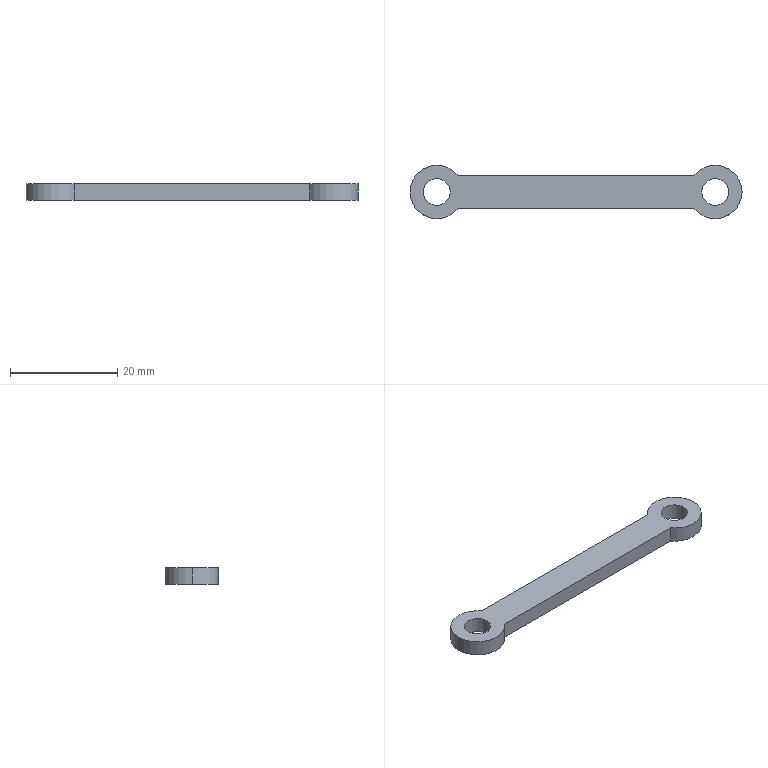Part | SolidWorks | features Extrusion 1 | 1 solid | 11 faces | box 62 x 10 x 3 mm | volume 1121 mm3 | cylinder 7 | plane 4 | commonest cylinder face diameters 5 x4 10 x3
STEP:
#1=CARTESIAN_POINT('',(49.5,0.,3.));
#2=VERTEX_POINT('',#1);
#3=CARTESIAN_POINT('',(54.5,0.,3.));
#4=VERTEX_POINT('',#3);
#5=CARTESIAN_POINT('',(52.,0.,3.));
#6=DIRECTION('',(0.,0.,1.));
#7=DIRECTION('',(1.,0.,0.));
#8=AXIS2_PLACEMENT_3D('',#5,#6,#7);
#9=CIRCLE('',#8,2.5);
#10=EDGE_CURVE('',#2,#4,#9,.T.);
#11=ORIENTED_EDGE('',*,*,#10,.T.);
#12=CARTESIAN_POINT('',(54.5,0.,0.));
#13=VERTEX_POINT('',#12);
#14=CARTESIAN_POINT('',(54.5,0.,3.));
#15=DIRECTION('',(0.,0.,-1.));
#16=VECTOR('',#15,1000.);
#17=LINE('',#14,#16);
#18=EDGE_CURVE('',#4,#13,#17,.T.);
#19=ORIENTED_EDGE('',*,*,#18,.T.);
#20=CARTESIAN_POINT('',(49.5,0.,0.));
#21=VERTEX_POINT('',#20);
#22=CARTESIAN_POINT('',(52.,0.,0.));
#23=DIRECTION('',(0.,0.,1.));
#24=DIRECTION('',(1.,0.,0.));
#25=AXIS2_PLACEMENT_3D('',#22,#23,#24);
#26=CIRCLE('',#25,2.5);
#27=EDGE_CURVE('',#21,#13,#26,.T.);
#28=ORIENTED_EDGE('',*,*,#27,.F.);
#29=CARTESIAN_POINT('',(49.5,0.,3.));
#30=DIRECTION('',(0.,0.,-1.));
#31=VECTOR('',#30,1000.);
#32=LINE('',#29,#31);
#33=EDGE_CURVE('',#2,#21,#32,.T.);
#34=ORIENTED_EDGE('',*,*,#33,.F.);
#35=EDGE_LOOP('',(#11,#19,#28,#34));
#36=FACE_OUTER_BOUND('',#35,.T.);
#37=CARTESIAN_POINT('',(52.,0.,3.));
#38=DIRECTION('',(0.,0.,-1.));
#39=DIRECTION('',(-1.,0.,0.));
#40=AXIS2_PLACEMENT_3D('',#37,#38,#39);
#41=CYLINDRICAL_SURFACE('',#40,2.5);
#42=ADVANCED_FACE('',(#36),#41,.F.);
#43=CARTESIAN_POINT('',(-2.5,0.,3.));
#44=VERTEX_POINT('',#43);
#45=CARTESIAN_POINT('',(2.5,0.,3.));
#46=VERTEX_POINT('',#45);
#47=CARTESIAN_POINT('',(0.,0.,3.));
#48=DIRECTION('',(0.,0.,1.));
#49=DIRECTION('',(1.,0.,0.));
#50=AXIS2_PLACEMENT_3D('',#47,#48,#49);
#51=CIRCLE('',#50,2.5);
#52=EDGE_CURVE('',#44,#46,#51,.T.);
#53=ORIENTED_EDGE('',*,*,#52,.T.);
#54=CARTESIAN_POINT('',(2.5,0.,0.));
#55=VERTEX_POINT('',#54);
#56=CARTESIAN_POINT('',(2.5,0.,3.));
#57=DIRECTION('',(0.,0.,-1.));
#58=VECTOR('',#57,1000.);
#59=LINE('',#56,#58);
#60=EDGE_CURVE('',#46,#55,#59,.T.);
#61=ORIENTED_EDGE('',*,*,#60,.T.);
#62=CARTESIAN_POINT('',(-2.5,0.,0.));
#63=VERTEX_POINT('',#62);
#64=CARTESIAN_POINT('',(0.,0.,0.));
#65=DIRECTION('',(0.,0.,1.));
#66=DIRECTION('',(1.,0.,0.));
#67=AXIS2_PLACEMENT_3D('',#64,#65,#66);
#68=CIRCLE('',#67,2.5);
#69=EDGE_CURVE('',#63,#55,#68,.T.);
#70=ORIENTED_EDGE('',*,*,#69,.F.);
#71=CARTESIAN_POINT('',(-2.5,0.,3.));
#72=DIRECTION('',(0.,0.,-1.));
#73=VECTOR('',#72,1000.);
#74=LINE('',#71,#73);
#75=EDGE_CURVE('',#44,#63,#74,.T.);
#76=ORIENTED_EDGE('',*,*,#75,.F.);
#77=EDGE_LOOP('',(#53,#61,#70,#76));
#78=FACE_OUTER_BOUND('',#77,.T.);
#79=CARTESIAN_POINT('',(0.,0.,3.));
#80=DIRECTION('',(0.,0.,-1.));
#81=DIRECTION('',(-1.,0.,0.));
#82=AXIS2_PLACEMENT_3D('',#79,#80,#81);
#83=CYLINDRICAL_SURFACE('',#82,2.5);
#84=ADVANCED_FACE('',(#78),#83,.F.);
#85=CARTESIAN_POINT('',(-5.,0.,3.));
#86=VERTEX_POINT('',#85);
#87=CARTESIAN_POINT('',(4.,-3.,3.));
#88=VERTEX_POINT('',#87);
#89=CARTESIAN_POINT('',(0.,0.,3.));
#90=DIRECTION('',(0.,0.,1.));
#91=DIRECTION('',(1.,0.,0.));
#92=AXIS2_PLACEMENT_3D('',#89,#90,#91);
#93=CIRCLE('',#92,5.);
#94=EDGE_CURVE('',#86,#88,#93,.T.);
#95=ORIENTED_EDGE('',*,*,#94,.F.);
#96=CARTESIAN_POINT('',(-5.,0.,0.));
#97=VERTEX_POINT('',#96);
#98=CARTESIAN_POINT('',(-5.,0.,3.));
#99=DIRECTION('',(0.,0.,-1.));
#100=VECTOR('',#99,1000.);
#101=LINE('',#98,#100);
#102=EDGE_CURVE('',#86,#97,#101,.T.);
#103=ORIENTED_EDGE('',*,*,#102,.T.);
#104=CARTESIAN_POINT('',(4.,-3.,0.));
#105=VERTEX_POINT('',#104);
#106=CARTESIAN_POINT('',(0.,0.,0.));
#107=DIRECTION('',(0.,0.,1.));
#108=DIRECTION('',(1.,0.,0.));
#109=AXIS2_PLACEMENT_3D('',#106,#107,#108);
#110=CIRCLE('',#109,5.);
#111=EDGE_CURVE('',#97,#105,#110,.T.);
#112=ORIENTED_EDGE('',*,*,#111,.T.);
#113=CARTESIAN_POINT('',(4.,-3.,3.));
#114=DIRECTION('',(0.,0.,-1.));
#115=VECTOR('',#114,1000.);
#116=LINE('',#113,#115);
#117=EDGE_CURVE('',#88,#105,#116,.T.);
#118=ORIENTED_EDGE('',*,*,#117,.F.);
#119=EDGE_LOOP('',(#95,#103,#112,#118));
#120=FACE_OUTER_BOUND('',#119,.T.);
#121=CARTESIAN_POINT('',(0.,0.,3.));
#122=DIRECTION('',(0.,0.,-1.));
#123=DIRECTION('',(-1.,0.,0.));
#124=AXIS2_PLACEMENT_3D('',#121,#122,#123);
#125=CYLINDRICAL_SURFACE('',#124,5.);
#126=ADVANCED_FACE('',(#120),#125,.T.);
#127=ORIENTED_EDGE('',*,*,#52,.F.);
#128=CARTESIAN_POINT('',(0.,0.,3.));
#129=DIRECTION('',(0.,0.,1.));
#130=DIRECTION('',(1.,0.,0.));
#131=AXIS2_PLACEMENT_3D('',#128,#129,#130);
#132=CIRCLE('',#131,2.5);
#133=EDGE_CURVE('',#46,#44,#132,.T.);
#134=ORIENTED_EDGE('',*,*,#133,.F.);
#135=EDGE_LOOP('',(#127,#134));
#136=FACE_BOUND('',#135,.T.);
#137=CARTESIAN_POINT('',(48.,-3.,3.));
#138=VERTEX_POINT('',#137);
#139=CARTESIAN_POINT('',(48.,3.,3.));
#140=VERTEX_POINT('',#139);
#141=CARTESIAN_POINT('',(52.,0.,3.));
#142=DIRECTION('',(0.,0.,1.));
#143=DIRECTION('',(1.,0.,0.));
#144=AXIS2_PLACEMENT_3D('',#141,#142,#143);
#145=CIRCLE('',#144,5.);
#146=EDGE_CURVE('',#138,#140,#145,.T.);
#147=ORIENTED_EDGE('',*,*,#146,.T.);
#148=CARTESIAN_POINT('',(4.,3.,3.));
#149=VERTEX_POINT('',#148);
#150=CARTESIAN_POINT('',(4.,3.,3.));
#151=DIRECTION('',(-1.,0.,0.));
#152=VECTOR('',#151,1000.);
#153=LINE('',#150,#152);
#154=EDGE_CURVE('',#140,#149,#153,.T.);
#155=ORIENTED_EDGE('',*,*,#154,.T.);
#156=CARTESIAN_POINT('',(0.,0.,3.));
#157=DIRECTION('',(0.,0.,1.));
#158=DIRECTION('',(1.,0.,0.));
#159=AXIS2_PLACEMENT_3D('',#156,#157,#158);
#160=CIRCLE('',#159,5.);
#161=EDGE_CURVE('',#149,#86,#160,.T.);
#162=ORIENTED_EDGE('',*,*,#161,.T.);
#163=ORIENTED_EDGE('',*,*,#94,.T.);
#164=CARTESIAN_POINT('',(4.,-3.,3.));
#165=DIRECTION('',(1.,0.,0.));
#166=VECTOR('',#165,1000.);
#167=LINE('',#164,#166);
#168=EDGE_CURVE('',#88,#138,#167,.T.);
#169=ORIENTED_EDGE('',*,*,#168,.T.);
#170=EDGE_LOOP('',(#147,#155,#162,#163,#169));
#171=FACE_OUTER_BOUND('',#170,.T.);
#172=ORIENTED_EDGE('',*,*,#10,.F.);
#173=CARTESIAN_POINT('',(52.,0.,3.));
#174=DIRECTION('',(0.,0.,1.));
#175=DIRECTION('',(1.,0.,0.));
#176=AXIS2_PLACEMENT_3D('',#173,#174,#175);
#177=CIRCLE('',#176,2.5);
#178=EDGE_CURVE('',#4,#2,#177,.T.);
#179=ORIENTED_EDGE('',*,*,#178,.F.);
#180=EDGE_LOOP('',(#172,#179));
#181=FACE_BOUND('',#180,.T.);
#182=CARTESIAN_POINT('',(52.,0.,3.));
#183=DIRECTION('',(0.,0.,1.));
#184=DIRECTION('',(1.,0.,0.));
#185=AXIS2_PLACEMENT_3D('',#182,#183,#184);
#186=PLANE('',#185);
#187=ADVANCED_FACE('',(#136,#171,#181),#186,.T.);
#188=CARTESIAN_POINT('',(48.,-3.,0.));
#189=VERTEX_POINT('',#188);
#190=CARTESIAN_POINT('',(48.,3.,0.));
#191=VERTEX_POINT('',#190);
#192=CARTESIAN_POINT('',(52.,0.,0.));
#193=DIRECTION('',(0.,0.,1.));
#194=DIRECTION('',(1.,0.,0.));
#195=AXIS2_PLACEMENT_3D('',#192,#193,#194);
#196=CIRCLE('',#195,5.);
#197=EDGE_CURVE('',#189,#191,#196,.T.);
#198=ORIENTED_EDGE('',*,*,#197,.F.);
#199=CARTESIAN_POINT('',(4.,-3.,0.));
#200=DIRECTION('',(1.,0.,0.));
#201=VECTOR('',#200,1000.);
#202=LINE('',#199,#201);
#203=EDGE_CURVE('',#105,#189,#202,.T.);
#204=ORIENTED_EDGE('',*,*,#203,.F.);
#205=ORIENTED_EDGE('',*,*,#111,.F.);
#206=CARTESIAN_POINT('',(4.,3.,0.));
#207=VERTEX_POINT('',#206);
#208=CARTESIAN_POINT('',(0.,0.,0.));
#209=DIRECTION('',(0.,0.,1.));
#210=DIRECTION('',(1.,0.,0.));
#211=AXIS2_PLACEMENT_3D('',#208,#209,#210);
#212=CIRCLE('',#211,5.);
#213=EDGE_CURVE('',#207,#97,#212,.T.);
#214=ORIENTED_EDGE('',*,*,#213,.F.);
#215=CARTESIAN_POINT('',(4.,3.,0.));
#216=DIRECTION('',(-1.,0.,0.));
#217=VECTOR('',#216,1000.);
#218=LINE('',#215,#217);
#219=EDGE_CURVE('',#191,#207,#218,.T.);
#220=ORIENTED_EDGE('',*,*,#219,.F.);
#221=EDGE_LOOP('',(#198,#204,#205,#214,#220));
#222=FACE_OUTER_BOUND('',#221,.T.);
#223=ORIENTED_EDGE('',*,*,#69,.T.);
#224=CARTESIAN_POINT('',(0.,0.,0.));
#225=DIRECTION('',(0.,0.,1.));
#226=DIRECTION('',(1.,0.,0.));
#227=AXIS2_PLACEMENT_3D('',#224,#225,#226);
#228=CIRCLE('',#227,2.5);
#229=EDGE_CURVE('',#55,#63,#228,.T.);
#230=ORIENTED_EDGE('',*,*,#229,.T.);
#231=EDGE_LOOP('',(#223,#230));
#232=FACE_BOUND('',#231,.T.);
#233=ORIENTED_EDGE('',*,*,#27,.T.);
#234=CARTESIAN_POINT('',(52.,0.,0.));
#235=DIRECTION('',(0.,0.,1.));
#236=DIRECTION('',(1.,0.,0.));
#237=AXIS2_PLACEMENT_3D('',#234,#235,#236);
#238=CIRCLE('',#237,2.5);
#239=EDGE_CURVE('',#13,#21,#238,.T.);
#240=ORIENTED_EDGE('',*,*,#239,.T.);
#241=EDGE_LOOP('',(#233,#240));
#242=FACE_BOUND('',#241,.T.);
#243=CARTESIAN_POINT('',(52.,0.,0.));
#244=DIRECTION('',(0.,0.,1.));
#245=DIRECTION('',(1.,0.,0.));
#246=AXIS2_PLACEMENT_3D('',#243,#244,#245);
#247=PLANE('',#246);
#248=ADVANCED_FACE('',(#222,#232,#242),#247,.F.);
#249=ORIENTED_EDGE('',*,*,#197,.T.);
#250=CARTESIAN_POINT('',(48.,3.,3.));
#251=DIRECTION('',(0.,0.,-1.));
#252=VECTOR('',#251,1000.);
#253=LINE('',#250,#252);
#254=EDGE_CURVE('',#140,#191,#253,.T.);
#255=ORIENTED_EDGE('',*,*,#254,.F.);
#256=ORIENTED_EDGE('',*,*,#146,.F.);
#257=CARTESIAN_POINT('',(48.,-3.,3.));
#258=DIRECTION('',(0.,0.,-1.));
#259=VECTOR('',#258,1000.);
#260=LINE('',#257,#259);
#261=EDGE_CURVE('',#138,#189,#260,.T.);
#262=ORIENTED_EDGE('',*,*,#261,.T.);
#263=EDGE_LOOP('',(#249,#255,#256,#262));
#264=FACE_OUTER_BOUND('',#263,.T.);
#265=CARTESIAN_POINT('',(52.,0.,3.));
#266=DIRECTION('',(0.,0.,-1.));
#267=DIRECTION('',(-1.,0.,0.));
#268=AXIS2_PLACEMENT_3D('',#265,#266,#267);
#269=CYLINDRICAL_SURFACE('',#268,5.);
#270=ADVANCED_FACE('',(#264),#269,.T.);
#271=ORIENTED_EDGE('',*,*,#219,.T.);
#272=CARTESIAN_POINT('',(4.,3.,3.));
#273=DIRECTION('',(0.,0.,-1.));
#274=VECTOR('',#273,1000.);
#275=LINE('',#272,#274);
#276=EDGE_CURVE('',#149,#207,#275,.T.);
#277=ORIENTED_EDGE('',*,*,#276,.F.);
#278=ORIENTED_EDGE('',*,*,#154,.F.);
#279=ORIENTED_EDGE('',*,*,#254,.T.);
#280=EDGE_LOOP('',(#271,#277,#278,#279));
#281=FACE_OUTER_BOUND('',#280,.T.);
#282=CARTESIAN_POINT('',(4.,3.,3.));
#283=DIRECTION('',(0.,-1.,0.));
#284=DIRECTION('',(0.,0.,-1.));
#285=AXIS2_PLACEMENT_3D('',#282,#283,#284);
#286=PLANE('',#285);
#287=ADVANCED_FACE('',(#281),#286,.F.);
#288=ORIENTED_EDGE('',*,*,#102,.F.);
#289=ORIENTED_EDGE('',*,*,#161,.F.);
#290=ORIENTED_EDGE('',*,*,#276,.T.);
#291=ORIENTED_EDGE('',*,*,#213,.T.);
#292=EDGE_LOOP('',(#288,#289,#290,#291));
#293=FACE_OUTER_BOUND('',#292,.T.);
#294=CARTESIAN_POINT('',(0.,0.,3.));
#295=DIRECTION('',(0.,0.,-1.));
#296=DIRECTION('',(-1.,0.,0.));
#297=AXIS2_PLACEMENT_3D('',#294,#295,#296);
#298=CYLINDRICAL_SURFACE('',#297,5.);
#299=ADVANCED_FACE('',(#293),#298,.T.);
#300=ORIENTED_EDGE('',*,*,#203,.T.);
#301=ORIENTED_EDGE('',*,*,#261,.F.);
#302=ORIENTED_EDGE('',*,*,#168,.F.);
#303=ORIENTED_EDGE('',*,*,#117,.T.);
#304=EDGE_LOOP('',(#300,#301,#302,#303));
#305=FACE_OUTER_BOUND('',#304,.T.);
#306=CARTESIAN_POINT('',(4.,-3.,3.));
#307=DIRECTION('',(0.,1.,0.));
#308=DIRECTION('',(0.,0.,1.));
#309=AXIS2_PLACEMENT_3D('',#306,#307,#308);
#310=PLANE('',#309);
#311=ADVANCED_FACE('',(#305),#310,.F.);
#312=ORIENTED_EDGE('',*,*,#60,.F.);
#313=ORIENTED_EDGE('',*,*,#133,.T.);
#314=ORIENTED_EDGE('',*,*,#75,.T.);
#315=ORIENTED_EDGE('',*,*,#229,.F.);
#316=EDGE_LOOP('',(#312,#313,#314,#315));
#317=FACE_OUTER_BOUND('',#316,.T.);
#318=CARTESIAN_POINT('',(0.,0.,3.));
#319=DIRECTION('',(0.,0.,-1.));
#320=DIRECTION('',(-1.,0.,0.));
#321=AXIS2_PLACEMENT_3D('',#318,#319,#320);
#322=CYLINDRICAL_SURFACE('',#321,2.5);
#323=ADVANCED_FACE('',(#317),#322,.F.);
#324=ORIENTED_EDGE('',*,*,#18,.F.);
#325=ORIENTED_EDGE('',*,*,#178,.T.);
#326=ORIENTED_EDGE('',*,*,#33,.T.);
#327=ORIENTED_EDGE('',*,*,#239,.F.);
#328=EDGE_LOOP('',(#324,#325,#326,#327));
#329=FACE_OUTER_BOUND('',#328,.T.);
#330=CARTESIAN_POINT('',(52.,0.,3.));
#331=DIRECTION('',(0.,0.,-1.));
#332=DIRECTION('',(-1.,0.,0.));
#333=AXIS2_PLACEMENT_3D('',#330,#331,#332);
#334=CYLINDRICAL_SURFACE('',#333,2.5);
#335=ADVANCED_FACE('',(#329),#334,.F.);
#336=CLOSED_SHELL('',(#42,#84,#126,#187,#248,#270,#287,#299,#311,#323,#335));
#337=MANIFOLD_SOLID_BREP('',#336);
#338=CARTESIAN_POINT('',(0.,0.,0.));
#339=DIRECTION('',(0.,0.,1.));
#340=DIRECTION('',(1.,0.,0.));
#341=AXIS2_PLACEMENT_3D('',#338,#339,#340);
#342=(LENGTH_UNIT()NAMED_UNIT(*)SI_UNIT(.MILLI.,.METRE.));
#343=UNCERTAINTY_MEASURE_WITH_UNIT(LENGTH_MEASURE(0.00001),#342,'','');
#344=(NAMED_UNIT(*)PLANE_ANGLE_UNIT()SI_UNIT($,.RADIAN.));
#345=(NAMED_UNIT(*)SI_UNIT($,.STERADIAN.)SOLID_ANGLE_UNIT());
#346=(GEOMETRIC_REPRESENTATION_CONTEXT(3)GLOBAL_UNCERTAINTY_ASSIGNED_CONTEXT((#343))GLOBAL_UNIT_ASSIGNED_CONTEXT((#342,#344,#345))REPRESENTATION_CONTEXT('',''));
#347=ADVANCED_BREP_SHAPE_REPRESENTATION('',(#337,#341),#346);